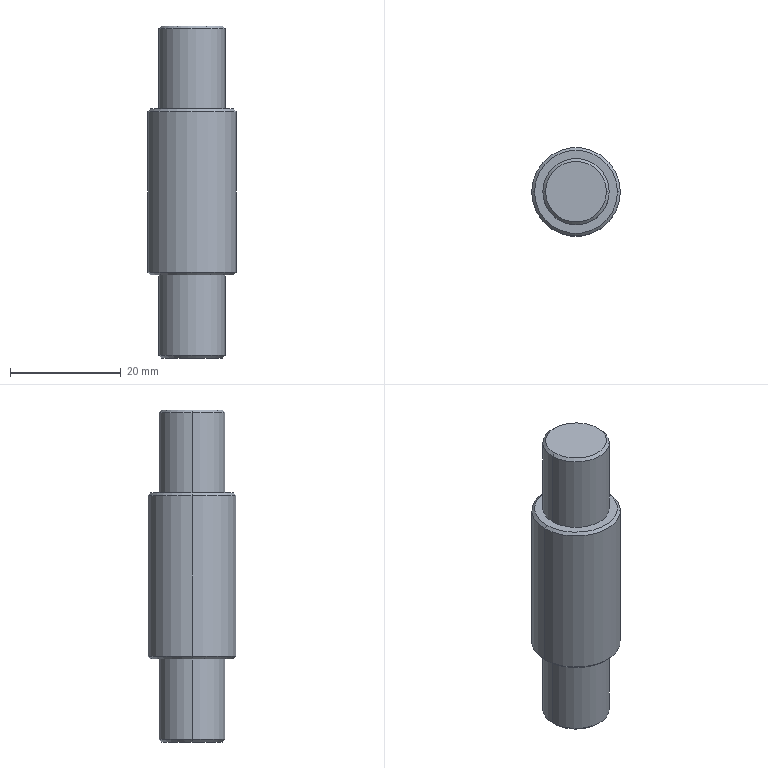Part | SolidWorks | features ICE 2, Chamfer 1, Extrusion 1 | 1 solid | 18 faces | box 16 x 16 x 60 mm | volume 9403 mm3 | cone 8 | cylinder 6 | plane 4 | commonest cylinder face diameters 12 x4 16 x2
STEP:
#1=CARTESIAN_POINT('',(7.5,0.,0.));
#2=VERTEX_POINT('',#1);
#3=CARTESIAN_POINT('',(-7.5,0.,0.));
#4=VERTEX_POINT('',#3);
#5=CARTESIAN_POINT('',(0.,0.,0.));
#6=DIRECTION('',(0.,0.,1.));
#7=DIRECTION('',(-1.,0.,0.));
#8=AXIS2_PLACEMENT_3D('',#5,#6,#7);
#9=CIRCLE('',#8,7.5);
#10=EDGE_CURVE('',#2,#4,#9,.T.);
#11=ORIENTED_EDGE('',*,*,#10,.F.);
#12=CARTESIAN_POINT('',(8.,0.,-0.5));
#13=VERTEX_POINT('',#12);
#14=CARTESIAN_POINT('',(8.,0.,-0.5));
#15=DIRECTION('',(0.7071,0.,-0.7071));
#16=VECTOR('',#15,1000.);
#17=LINE('',#14,#16);
#18=EDGE_CURVE('',#2,#13,#17,.T.);
#19=ORIENTED_EDGE('',*,*,#18,.T.);
#20=CARTESIAN_POINT('',(-8.,0.,-0.5));
#21=VERTEX_POINT('',#20);
#22=CARTESIAN_POINT('',(0.,0.,-0.5));
#23=DIRECTION('',(0.,0.,-1.));
#24=DIRECTION('',(-1.,0.,0.));
#25=AXIS2_PLACEMENT_3D('',#22,#23,#24);
#26=CIRCLE('',#25,8.);
#27=EDGE_CURVE('',#21,#13,#26,.T.);
#28=ORIENTED_EDGE('',*,*,#27,.F.);
#29=CARTESIAN_POINT('',(-8.,0.,-0.5));
#30=DIRECTION('',(-0.7071,0.,-0.7071));
#31=VECTOR('',#30,1000.);
#32=LINE('',#29,#31);
#33=EDGE_CURVE('',#4,#21,#32,.T.);
#34=ORIENTED_EDGE('',*,*,#33,.F.);
#35=EDGE_LOOP('',(#11,#19,#28,#34));
#36=FACE_OUTER_BOUND('',#35,.T.);
#37=CARTESIAN_POINT('',(0.,0.,-0.5));
#38=DIRECTION('',(0.,0.,-1.));
#39=DIRECTION('',(-1.,0.,0.));
#40=AXIS2_PLACEMENT_3D('',#37,#38,#39);
#41=CONICAL_SURFACE('',#40,8.,0.7854);
#42=ADVANCED_FACE('',(#36),#41,.T.);
#43=CARTESIAN_POINT('',(-7.5,0.,-30.));
#44=VERTEX_POINT('',#43);
#45=CARTESIAN_POINT('',(7.5,0.,-30.));
#46=VERTEX_POINT('',#45);
#47=CARTESIAN_POINT('',(0.,0.,-30.));
#48=DIRECTION('',(0.,0.,-1.));
#49=DIRECTION('',(-1.,0.,0.));
#50=AXIS2_PLACEMENT_3D('',#47,#48,#49);
#51=CIRCLE('',#50,7.5);
#52=EDGE_CURVE('',#44,#46,#51,.T.);
#53=ORIENTED_EDGE('',*,*,#52,.F.);
#54=CARTESIAN_POINT('',(-8.,0.,-29.5));
#55=VERTEX_POINT('',#54);
#56=CARTESIAN_POINT('',(-7.5,0.,-30.));
#57=DIRECTION('',(-0.7071,0.,0.7071));
#58=VECTOR('',#57,1000.);
#59=LINE('',#56,#58);
#60=EDGE_CURVE('',#44,#55,#59,.T.);
#61=ORIENTED_EDGE('',*,*,#60,.T.);
#62=CARTESIAN_POINT('',(8.,0.,-29.5));
#63=VERTEX_POINT('',#62);
#64=CARTESIAN_POINT('',(0.,0.,-29.5));
#65=DIRECTION('',(0.,0.,1.));
#66=DIRECTION('',(-1.,0.,0.));
#67=AXIS2_PLACEMENT_3D('',#64,#65,#66);
#68=CIRCLE('',#67,8.);
#69=EDGE_CURVE('',#63,#55,#68,.T.);
#70=ORIENTED_EDGE('',*,*,#69,.F.);
#71=CARTESIAN_POINT('',(7.5,0.,-30.));
#72=DIRECTION('',(0.7071,0.,0.7071));
#73=VECTOR('',#72,1000.);
#74=LINE('',#71,#73);
#75=EDGE_CURVE('',#46,#63,#74,.T.);
#76=ORIENTED_EDGE('',*,*,#75,.F.);
#77=EDGE_LOOP('',(#53,#61,#70,#76));
#78=FACE_OUTER_BOUND('',#77,.T.);
#79=CARTESIAN_POINT('',(0.,0.,-30.));
#80=DIRECTION('',(0.,0.,1.));
#81=DIRECTION('',(1.,0.,0.));
#82=AXIS2_PLACEMENT_3D('',#79,#80,#81);
#83=CONICAL_SURFACE('',#82,7.5,0.7854);
#84=ADVANCED_FACE('',(#78),#83,.T.);
#85=CARTESIAN_POINT('',(-5.5,0.,-45.));
#86=VERTEX_POINT('',#85);
#87=CARTESIAN_POINT('',(5.5,0.,-45.));
#88=VERTEX_POINT('',#87);
#89=CARTESIAN_POINT('',(0.,0.,-45.));
#90=DIRECTION('',(0.,0.,-1.));
#91=DIRECTION('',(-1.,0.,0.));
#92=AXIS2_PLACEMENT_3D('',#89,#90,#91);
#93=CIRCLE('',#92,5.5);
#94=EDGE_CURVE('',#86,#88,#93,.T.);
#95=ORIENTED_EDGE('',*,*,#94,.F.);
#96=CARTESIAN_POINT('',(-6.,0.,-44.5));
#97=VERTEX_POINT('',#96);
#98=CARTESIAN_POINT('',(-5.5,0.,-45.));
#99=DIRECTION('',(-0.7071,0.,0.7071));
#100=VECTOR('',#99,1000.);
#101=LINE('',#98,#100);
#102=EDGE_CURVE('',#86,#97,#101,.T.);
#103=ORIENTED_EDGE('',*,*,#102,.T.);
#104=CARTESIAN_POINT('',(6.,0.,-44.5));
#105=VERTEX_POINT('',#104);
#106=CARTESIAN_POINT('',(0.,0.,-44.5));
#107=DIRECTION('',(0.,0.,1.));
#108=DIRECTION('',(-1.,0.,0.));
#109=AXIS2_PLACEMENT_3D('',#106,#107,#108);
#110=CIRCLE('',#109,6.);
#111=EDGE_CURVE('',#105,#97,#110,.T.);
#112=ORIENTED_EDGE('',*,*,#111,.F.);
#113=CARTESIAN_POINT('',(5.5,0.,-45.));
#114=DIRECTION('',(0.7071,0.,0.7071));
#115=VECTOR('',#114,1000.);
#116=LINE('',#113,#115);
#117=EDGE_CURVE('',#88,#105,#116,.T.);
#118=ORIENTED_EDGE('',*,*,#117,.F.);
#119=EDGE_LOOP('',(#95,#103,#112,#118));
#120=FACE_OUTER_BOUND('',#119,.T.);
#121=CARTESIAN_POINT('',(0.,0.,-45.));
#122=DIRECTION('',(0.,0.,1.));
#123=DIRECTION('',(1.,0.,0.));
#124=AXIS2_PLACEMENT_3D('',#121,#122,#123);
#125=CONICAL_SURFACE('',#124,5.5,0.7854);
#126=ADVANCED_FACE('',(#120),#125,.T.);
#127=CARTESIAN_POINT('',(5.5,0.,15.));
#128=VERTEX_POINT('',#127);
#129=CARTESIAN_POINT('',(-5.5,0.,15.));
#130=VERTEX_POINT('',#129);
#131=CARTESIAN_POINT('',(0.,0.,15.));
#132=DIRECTION('',(0.,0.,1.));
#133=DIRECTION('',(1.,0.,0.));
#134=AXIS2_PLACEMENT_3D('',#131,#132,#133);
#135=CIRCLE('',#134,5.5);
#136=EDGE_CURVE('',#128,#130,#135,.T.);
#137=ORIENTED_EDGE('',*,*,#136,.F.);
#138=CARTESIAN_POINT('',(6.,0.,14.5));
#139=VERTEX_POINT('',#138);
#140=CARTESIAN_POINT('',(5.5,0.,15.));
#141=DIRECTION('',(0.7071,0.,-0.7071));
#142=VECTOR('',#141,1000.);
#143=LINE('',#140,#142);
#144=EDGE_CURVE('',#128,#139,#143,.T.);
#145=ORIENTED_EDGE('',*,*,#144,.T.);
#146=CARTESIAN_POINT('',(-6.,0.,14.5));
#147=VERTEX_POINT('',#146);
#148=CARTESIAN_POINT('',(0.,0.,14.5));
#149=DIRECTION('',(0.,0.,-1.));
#150=DIRECTION('',(1.,0.,0.));
#151=AXIS2_PLACEMENT_3D('',#148,#149,#150);
#152=CIRCLE('',#151,6.);
#153=EDGE_CURVE('',#147,#139,#152,.T.);
#154=ORIENTED_EDGE('',*,*,#153,.F.);
#155=CARTESIAN_POINT('',(-5.5,0.,15.));
#156=DIRECTION('',(-0.7071,0.,-0.7071));
#157=VECTOR('',#156,1000.);
#158=LINE('',#155,#157);
#159=EDGE_CURVE('',#130,#147,#158,.T.);
#160=ORIENTED_EDGE('',*,*,#159,.F.);
#161=EDGE_LOOP('',(#137,#145,#154,#160));
#162=FACE_OUTER_BOUND('',#161,.T.);
#163=CARTESIAN_POINT('',(0.,0.,15.));
#164=DIRECTION('',(0.,0.,-1.));
#165=DIRECTION('',(-1.,0.,0.));
#166=AXIS2_PLACEMENT_3D('',#163,#164,#165);
#167=CONICAL_SURFACE('',#166,5.5,0.7854);
#168=ADVANCED_FACE('',(#162),#167,.T.);
#169=ORIENTED_EDGE('',*,*,#111,.T.);
#170=CARTESIAN_POINT('',(-6.,0.,-30.));
#171=VERTEX_POINT('',#170);
#172=CARTESIAN_POINT('',(-6.,0.,-45.));
#173=DIRECTION('',(0.,0.,1.));
#174=VECTOR('',#173,1000.);
#175=LINE('',#172,#174);
#176=EDGE_CURVE('',#97,#171,#175,.T.);
#177=ORIENTED_EDGE('',*,*,#176,.T.);
#178=CARTESIAN_POINT('',(6.,0.,-30.));
#179=VERTEX_POINT('',#178);
#180=CARTESIAN_POINT('',(0.,0.,-30.));
#181=DIRECTION('',(0.,0.,-1.));
#182=DIRECTION('',(-1.,0.,0.));
#183=AXIS2_PLACEMENT_3D('',#180,#181,#182);
#184=CIRCLE('',#183,6.);
#185=EDGE_CURVE('',#171,#179,#184,.T.);
#186=ORIENTED_EDGE('',*,*,#185,.T.);
#187=CARTESIAN_POINT('',(6.,0.,-45.));
#188=DIRECTION('',(0.,0.,1.));
#189=VECTOR('',#188,1000.);
#190=LINE('',#187,#189);
#191=EDGE_CURVE('',#105,#179,#190,.T.);
#192=ORIENTED_EDGE('',*,*,#191,.F.);
#193=EDGE_LOOP('',(#169,#177,#186,#192));
#194=FACE_OUTER_BOUND('',#193,.T.);
#195=CARTESIAN_POINT('',(0.,0.,-45.));
#196=DIRECTION('',(0.,0.,1.));
#197=DIRECTION('',(1.,0.,0.));
#198=AXIS2_PLACEMENT_3D('',#195,#196,#197);
#199=CYLINDRICAL_SURFACE('',#198,6.);
#200=ADVANCED_FACE('',(#194),#199,.T.);
#201=ORIENTED_EDGE('',*,*,#69,.T.);
#202=CARTESIAN_POINT('',(-8.,0.,-30.));
#203=DIRECTION('',(0.,0.,1.));
#204=VECTOR('',#203,1000.);
#205=LINE('',#202,#204);
#206=EDGE_CURVE('',#55,#21,#205,.T.);
#207=ORIENTED_EDGE('',*,*,#206,.T.);
#208=ORIENTED_EDGE('',*,*,#27,.T.);
#209=CARTESIAN_POINT('',(8.,0.,-30.));
#210=DIRECTION('',(0.,0.,1.));
#211=VECTOR('',#210,1000.);
#212=LINE('',#209,#211);
#213=EDGE_CURVE('',#63,#13,#212,.T.);
#214=ORIENTED_EDGE('',*,*,#213,.F.);
#215=EDGE_LOOP('',(#201,#207,#208,#214));
#216=FACE_OUTER_BOUND('',#215,.T.);
#217=CARTESIAN_POINT('',(0.,0.,-30.));
#218=DIRECTION('',(0.,0.,1.));
#219=DIRECTION('',(1.,0.,0.));
#220=AXIS2_PLACEMENT_3D('',#217,#218,#219);
#221=CYLINDRICAL_SURFACE('',#220,8.);
#222=ADVANCED_FACE('',(#216),#221,.T.);
#223=ORIENTED_EDGE('',*,*,#153,.T.);
#224=CARTESIAN_POINT('',(6.,0.,0.));
#225=VERTEX_POINT('',#224);
#226=CARTESIAN_POINT('',(6.,0.,15.));
#227=DIRECTION('',(0.,0.,-1.));
#228=VECTOR('',#227,1000.);
#229=LINE('',#226,#228);
#230=EDGE_CURVE('',#139,#225,#229,.T.);
#231=ORIENTED_EDGE('',*,*,#230,.T.);
#232=CARTESIAN_POINT('',(-6.,0.,0.));
#233=VERTEX_POINT('',#232);
#234=CARTESIAN_POINT('',(0.,0.,0.));
#235=DIRECTION('',(0.,0.,1.));
#236=DIRECTION('',(1.,0.,0.));
#237=AXIS2_PLACEMENT_3D('',#234,#235,#236);
#238=CIRCLE('',#237,6.);
#239=EDGE_CURVE('',#225,#233,#238,.T.);
#240=ORIENTED_EDGE('',*,*,#239,.T.);
#241=CARTESIAN_POINT('',(-6.,0.,15.));
#242=DIRECTION('',(0.,0.,-1.));
#243=VECTOR('',#242,1000.);
#244=LINE('',#241,#243);
#245=EDGE_CURVE('',#147,#233,#244,.T.);
#246=ORIENTED_EDGE('',*,*,#245,.F.);
#247=EDGE_LOOP('',(#223,#231,#240,#246));
#248=FACE_OUTER_BOUND('',#247,.T.);
#249=CARTESIAN_POINT('',(0.,0.,15.));
#250=DIRECTION('',(0.,0.,-1.));
#251=DIRECTION('',(-1.,0.,0.));
#252=AXIS2_PLACEMENT_3D('',#249,#250,#251);
#253=CYLINDRICAL_SURFACE('',#252,6.);
#254=ADVANCED_FACE('',(#248),#253,.T.);
#255=ORIENTED_EDGE('',*,*,#230,.F.);
#256=CARTESIAN_POINT('',(0.,0.,14.5));
#257=DIRECTION('',(0.,0.,-1.));
#258=DIRECTION('',(1.,0.,0.));
#259=AXIS2_PLACEMENT_3D('',#256,#257,#258);
#260=CIRCLE('',#259,6.);
#261=EDGE_CURVE('',#139,#147,#260,.T.);
#262=ORIENTED_EDGE('',*,*,#261,.T.);
#263=ORIENTED_EDGE('',*,*,#245,.T.);
#264=CARTESIAN_POINT('',(0.,0.,0.));
#265=DIRECTION('',(0.,0.,1.));
#266=DIRECTION('',(1.,0.,0.));
#267=AXIS2_PLACEMENT_3D('',#264,#265,#266);
#268=CIRCLE('',#267,6.);
#269=EDGE_CURVE('',#233,#225,#268,.T.);
#270=ORIENTED_EDGE('',*,*,#269,.T.);
#271=EDGE_LOOP('',(#255,#262,#263,#270));
#272=FACE_OUTER_BOUND('',#271,.T.);
#273=CARTESIAN_POINT('',(0.,0.,15.));
#274=DIRECTION('',(0.,0.,-1.));
#275=DIRECTION('',(-1.,0.,0.));
#276=AXIS2_PLACEMENT_3D('',#273,#274,#275);
#277=CYLINDRICAL_SURFACE('',#276,6.);
#278=ADVANCED_FACE('',(#272),#277,.T.);
#279=CARTESIAN_POINT('',(0.,0.,15.));
#280=DIRECTION('',(0.,0.,1.));
#281=DIRECTION('',(1.,0.,0.));
#282=AXIS2_PLACEMENT_3D('',#279,#280,#281);
#283=CIRCLE('',#282,5.5);
#284=EDGE_CURVE('',#130,#128,#283,.T.);
#285=ORIENTED_EDGE('',*,*,#284,.T.);
#286=ORIENTED_EDGE('',*,*,#136,.T.);
#287=EDGE_LOOP('',(#285,#286));
#288=FACE_OUTER_BOUND('',#287,.T.);
#289=CARTESIAN_POINT('',(0.,0.,15.));
#290=DIRECTION('',(0.,0.,1.));
#291=DIRECTION('',(1.,0.,0.));
#292=AXIS2_PLACEMENT_3D('',#289,#290,#291);
#293=PLANE('',#292);
#294=ADVANCED_FACE('',(#288),#293,.T.);
#295=ORIENTED_EDGE('',*,*,#206,.F.);
#296=CARTESIAN_POINT('',(0.,0.,-29.5));
#297=DIRECTION('',(0.,0.,1.));
#298=DIRECTION('',(-1.,0.,0.));
#299=AXIS2_PLACEMENT_3D('',#296,#297,#298);
#300=CIRCLE('',#299,8.);
#301=EDGE_CURVE('',#55,#63,#300,.T.);
#302=ORIENTED_EDGE('',*,*,#301,.T.);
#303=ORIENTED_EDGE('',*,*,#213,.T.);
#304=CARTESIAN_POINT('',(0.,0.,-0.5));
#305=DIRECTION('',(0.,0.,-1.));
#306=DIRECTION('',(-1.,0.,0.));
#307=AXIS2_PLACEMENT_3D('',#304,#305,#306);
#308=CIRCLE('',#307,8.);
#309=EDGE_CURVE('',#13,#21,#308,.T.);
#310=ORIENTED_EDGE('',*,*,#309,.T.);
#311=EDGE_LOOP('',(#295,#302,#303,#310));
#312=FACE_OUTER_BOUND('',#311,.T.);
#313=CARTESIAN_POINT('',(0.,0.,-30.));
#314=DIRECTION('',(0.,0.,1.));
#315=DIRECTION('',(1.,0.,0.));
#316=AXIS2_PLACEMENT_3D('',#313,#314,#315);
#317=CYLINDRICAL_SURFACE('',#316,8.);
#318=ADVANCED_FACE('',(#312),#317,.T.);
#319=CARTESIAN_POINT('',(0.,0.,-30.));
#320=DIRECTION('',(0.,0.,-1.));
#321=DIRECTION('',(-1.,0.,0.));
#322=AXIS2_PLACEMENT_3D('',#319,#320,#321);
#323=CIRCLE('',#322,7.5);
#324=EDGE_CURVE('',#46,#44,#323,.T.);
#325=ORIENTED_EDGE('',*,*,#324,.T.);
#326=ORIENTED_EDGE('',*,*,#52,.T.);
#327=EDGE_LOOP('',(#325,#326));
#328=FACE_OUTER_BOUND('',#327,.T.);
#329=CARTESIAN_POINT('',(0.,0.,-30.));
#330=DIRECTION('',(0.,0.,-1.));
#331=DIRECTION('',(-1.,0.,0.));
#332=AXIS2_PLACEMENT_3D('',#329,#330,#331);
#333=CIRCLE('',#332,6.);
#334=EDGE_CURVE('',#179,#171,#333,.T.);
#335=ORIENTED_EDGE('',*,*,#334,.F.);
#336=ORIENTED_EDGE('',*,*,#185,.F.);
#337=EDGE_LOOP('',(#335,#336));
#338=FACE_BOUND('',#337,.T.);
#339=CARTESIAN_POINT('',(0.,0.,-30.));
#340=DIRECTION('',(0.,0.,-1.));
#341=DIRECTION('',(-1.,0.,0.));
#342=AXIS2_PLACEMENT_3D('',#339,#340,#341);
#343=PLANE('',#342);
#344=ADVANCED_FACE('',(#328,#338),#343,.T.);
#345=CARTESIAN_POINT('',(0.,0.,0.));
#346=DIRECTION('',(0.,0.,1.));
#347=DIRECTION('',(-1.,0.,0.));
#348=AXIS2_PLACEMENT_3D('',#345,#346,#347);
#349=CIRCLE('',#348,7.5);
#350=EDGE_CURVE('',#4,#2,#349,.T.);
#351=ORIENTED_EDGE('',*,*,#350,.T.);
#352=ORIENTED_EDGE('',*,*,#10,.T.);
#353=EDGE_LOOP('',(#351,#352));
#354=FACE_OUTER_BOUND('',#353,.T.);
#355=ORIENTED_EDGE('',*,*,#269,.F.);
#356=ORIENTED_EDGE('',*,*,#239,.F.);
#357=EDGE_LOOP('',(#355,#356));
#358=FACE_BOUND('',#357,.T.);
#359=CARTESIAN_POINT('',(0.,0.,0.));
#360=DIRECTION('',(0.,0.,-1.));
#361=DIRECTION('',(-1.,0.,0.));
#362=AXIS2_PLACEMENT_3D('',#359,#360,#361);
#363=PLANE('',#362);
#364=ADVANCED_FACE('',(#354,#358),#363,.F.);
#365=ORIENTED_EDGE('',*,*,#176,.F.);
#366=CARTESIAN_POINT('',(0.,0.,-44.5));
#367=DIRECTION('',(0.,0.,1.));
#368=DIRECTION('',(-1.,0.,0.));
#369=AXIS2_PLACEMENT_3D('',#366,#367,#368);
#370=CIRCLE('',#369,6.);
#371=EDGE_CURVE('',#97,#105,#370,.T.);
#372=ORIENTED_EDGE('',*,*,#371,.T.);
#373=ORIENTED_EDGE('',*,*,#191,.T.);
#374=ORIENTED_EDGE('',*,*,#334,.T.);
#375=EDGE_LOOP('',(#365,#372,#373,#374));
#376=FACE_OUTER_BOUND('',#375,.T.);
#377=CARTESIAN_POINT('',(0.,0.,-45.));
#378=DIRECTION('',(0.,0.,1.));
#379=DIRECTION('',(1.,0.,0.));
#380=AXIS2_PLACEMENT_3D('',#377,#378,#379);
#381=CYLINDRICAL_SURFACE('',#380,6.);
#382=ADVANCED_FACE('',(#376),#381,.T.);
#383=CARTESIAN_POINT('',(0.,0.,-45.));
#384=DIRECTION('',(0.,0.,-1.));
#385=DIRECTION('',(-1.,0.,0.));
#386=AXIS2_PLACEMENT_3D('',#383,#384,#385);
#387=CIRCLE('',#386,5.5);
#388=EDGE_CURVE('',#88,#86,#387,.T.);
#389=ORIENTED_EDGE('',*,*,#388,.T.);
#390=ORIENTED_EDGE('',*,*,#94,.T.);
#391=EDGE_LOOP('',(#389,#390));
#392=FACE_OUTER_BOUND('',#391,.T.);
#393=CARTESIAN_POINT('',(0.,0.,-45.));
#394=DIRECTION('',(0.,0.,-1.));
#395=DIRECTION('',(-1.,0.,0.));
#396=AXIS2_PLACEMENT_3D('',#393,#394,#395);
#397=PLANE('',#396);
#398=ADVANCED_FACE('',(#392),#397,.T.);
#399=ORIENTED_EDGE('',*,*,#144,.F.);
#400=ORIENTED_EDGE('',*,*,#284,.F.);
#401=ORIENTED_EDGE('',*,*,#159,.T.);
#402=ORIENTED_EDGE('',*,*,#261,.F.);
#403=EDGE_LOOP('',(#399,#400,#401,#402));
#404=FACE_OUTER_BOUND('',#403,.T.);
#405=CARTESIAN_POINT('',(0.,0.,15.));
#406=DIRECTION('',(0.,0.,-1.));
#407=DIRECTION('',(-1.,0.,0.));
#408=AXIS2_PLACEMENT_3D('',#405,#406,#407);
#409=CONICAL_SURFACE('',#408,5.5,0.7854);
#410=ADVANCED_FACE('',(#404),#409,.T.);
#411=ORIENTED_EDGE('',*,*,#102,.F.);
#412=ORIENTED_EDGE('',*,*,#388,.F.);
#413=ORIENTED_EDGE('',*,*,#117,.T.);
#414=ORIENTED_EDGE('',*,*,#371,.F.);
#415=EDGE_LOOP('',(#411,#412,#413,#414));
#416=FACE_OUTER_BOUND('',#415,.T.);
#417=CARTESIAN_POINT('',(0.,0.,-45.));
#418=DIRECTION('',(0.,0.,1.));
#419=DIRECTION('',(1.,0.,0.));
#420=AXIS2_PLACEMENT_3D('',#417,#418,#419);
#421=CONICAL_SURFACE('',#420,5.5,0.7854);
#422=ADVANCED_FACE('',(#416),#421,.T.);
#423=ORIENTED_EDGE('',*,*,#60,.F.);
#424=ORIENTED_EDGE('',*,*,#324,.F.);
#425=ORIENTED_EDGE('',*,*,#75,.T.);
#426=ORIENTED_EDGE('',*,*,#301,.F.);
#427=EDGE_LOOP('',(#423,#424,#425,#426));
#428=FACE_OUTER_BOUND('',#427,.T.);
#429=CARTESIAN_POINT('',(0.,0.,-30.));
#430=DIRECTION('',(0.,0.,1.));
#431=DIRECTION('',(1.,0.,0.));
#432=AXIS2_PLACEMENT_3D('',#429,#430,#431);
#433=CONICAL_SURFACE('',#432,7.5,0.7854);
#434=ADVANCED_FACE('',(#428),#433,.T.);
#435=ORIENTED_EDGE('',*,*,#18,.F.);
#436=ORIENTED_EDGE('',*,*,#350,.F.);
#437=ORIENTED_EDGE('',*,*,#33,.T.);
#438=ORIENTED_EDGE('',*,*,#309,.F.);
#439=EDGE_LOOP('',(#435,#436,#437,#438));
#440=FACE_OUTER_BOUND('',#439,.T.);
#441=CARTESIAN_POINT('',(0.,0.,-0.5));
#442=DIRECTION('',(0.,0.,-1.));
#443=DIRECTION('',(-1.,0.,0.));
#444=AXIS2_PLACEMENT_3D('',#441,#442,#443);
#445=CONICAL_SURFACE('',#444,8.,0.7854);
#446=ADVANCED_FACE('',(#440),#445,.T.);
#447=CLOSED_SHELL('',(#42,#84,#126,#168,#200,#222,#254,#278,#294,#318,#344,#364,#382,#398,#410,#422,#434,#446));
#448=MANIFOLD_SOLID_BREP('',#447);
#449=CARTESIAN_POINT('',(0.,0.,0.));
#450=DIRECTION('',(0.,0.,1.));
#451=DIRECTION('',(1.,0.,0.));
#452=AXIS2_PLACEMENT_3D('',#449,#450,#451);
#453=(LENGTH_UNIT()NAMED_UNIT(*)SI_UNIT(.MILLI.,.METRE.));
#454=UNCERTAINTY_MEASURE_WITH_UNIT(LENGTH_MEASURE(0.00001),#453,'','');
#455=(NAMED_UNIT(*)PLANE_ANGLE_UNIT()SI_UNIT($,.RADIAN.));
#456=(NAMED_UNIT(*)SI_UNIT($,.STERADIAN.)SOLID_ANGLE_UNIT());
#457=(GEOMETRIC_REPRESENTATION_CONTEXT(3)GLOBAL_UNCERTAINTY_ASSIGNED_CONTEXT((#454))GLOBAL_UNIT_ASSIGNED_CONTEXT((#453,#455,#456))REPRESENTATION_CONTEXT('',''));
#458=ADVANCED_BREP_SHAPE_REPRESENTATION('',(#448,#452),#457);